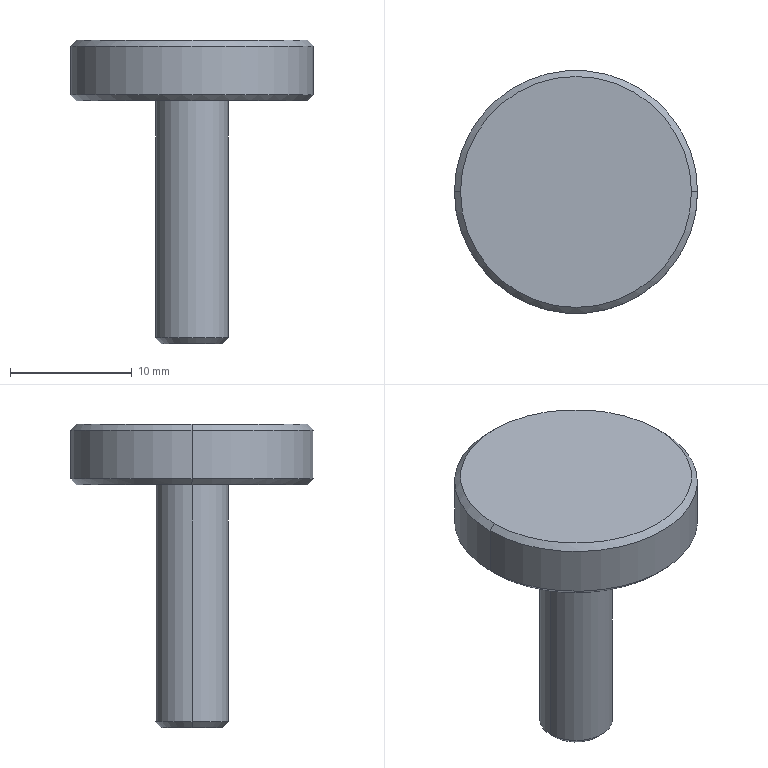Part | NX | features BREP 1 | 1 solid | 16 faces | box 20 x 20 x 25 mm | volume 2097 mm3 | cylinder 6 | cone 6 | plane 4 | commonest cylinder face diameters 3 x2 6 x2 20 x2
STEP:
#1=CARTESIAN_POINT('',(1.5,0.,3.));
#2=VERTEX_POINT('',#1);
#3=CARTESIAN_POINT('',(-1.5,0.,3.));
#4=VERTEX_POINT('',#3);
#5=CARTESIAN_POINT('',(0.,0.,3.));
#6=DIRECTION('',(0.,0.,-1.));
#7=DIRECTION('',(-1.,0.,0.));
#8=AXIS2_PLACEMENT_3D('',#5,#6,#7);
#9=CIRCLE('',#8,1.5);
#10=EDGE_CURVE('',#2,#4,#9,.T.);
#11=ORIENTED_EDGE('',*,*,#10,.F.);
#12=CARTESIAN_POINT('',(1.5,0.,0.));
#13=VERTEX_POINT('',#12);
#14=CARTESIAN_POINT('',(1.5,0.,3.));
#15=DIRECTION('',(0.,0.,-1.));
#16=VECTOR('',#15,1000.);
#17=LINE('',#14,#16);
#18=EDGE_CURVE('',#2,#13,#17,.T.);
#19=ORIENTED_EDGE('',*,*,#18,.T.);
#20=CARTESIAN_POINT('',(-1.5,0.,0.));
#21=VERTEX_POINT('',#20);
#22=CARTESIAN_POINT('',(0.,0.,0.));
#23=DIRECTION('',(0.,0.,-1.));
#24=DIRECTION('',(-1.,0.,0.));
#25=AXIS2_PLACEMENT_3D('',#22,#23,#24);
#26=CIRCLE('',#25,1.5);
#27=EDGE_CURVE('',#13,#21,#26,.T.);
#28=ORIENTED_EDGE('',*,*,#27,.T.);
#29=CARTESIAN_POINT('',(-1.5,0.,3.));
#30=DIRECTION('',(0.,0.,-1.));
#31=VECTOR('',#30,1000.);
#32=LINE('',#29,#31);
#33=EDGE_CURVE('',#4,#21,#32,.T.);
#34=ORIENTED_EDGE('',*,*,#33,.F.);
#35=EDGE_LOOP('',(#11,#19,#28,#34));
#36=FACE_BOUND('',#35,.T.);
#37=CARTESIAN_POINT('',(0.,0.,3.));
#38=DIRECTION('',(0.,0.,-1.));
#39=DIRECTION('',(-1.,0.,0.));
#40=AXIS2_PLACEMENT_3D('',#37,#38,#39);
#41=CYLINDRICAL_SURFACE('',#40,1.5);
#42=ADVANCED_FACE('',(#36),#41,.F.);
#43=CARTESIAN_POINT('',(-9.5,0.,20.));
#44=VERTEX_POINT('',#43);
#45=CARTESIAN_POINT('',(9.5,0.,20.));
#46=VERTEX_POINT('',#45);
#47=CARTESIAN_POINT('',(0.,0.,20.));
#48=DIRECTION('',(0.,0.,-1.));
#49=DIRECTION('',(1.,0.,0.));
#50=AXIS2_PLACEMENT_3D('',#47,#48,#49);
#51=CIRCLE('',#50,9.5);
#52=EDGE_CURVE('',#44,#46,#51,.T.);
#53=ORIENTED_EDGE('',*,*,#52,.F.);
#54=CARTESIAN_POINT('',(-10.,0.,20.5));
#55=VERTEX_POINT('',#54);
#56=CARTESIAN_POINT('',(-10.,0.,20.5));
#57=DIRECTION('',(-0.7071,0.,0.7071));
#58=VECTOR('',#57,1000.);
#59=LINE('',#56,#58);
#60=EDGE_CURVE('',#55,#44,#59,.F.);
#61=ORIENTED_EDGE('',*,*,#60,.F.);
#62=CARTESIAN_POINT('',(10.,0.,20.5));
#63=VERTEX_POINT('',#62);
#64=CARTESIAN_POINT('',(0.,0.,20.5));
#65=DIRECTION('',(0.,0.,1.));
#66=DIRECTION('',(1.,0.,0.));
#67=AXIS2_PLACEMENT_3D('',#64,#65,#66);
#68=CIRCLE('',#67,10.);
#69=EDGE_CURVE('',#63,#55,#68,.T.);
#70=ORIENTED_EDGE('',*,*,#69,.F.);
#71=CARTESIAN_POINT('',(10.,0.,20.5));
#72=DIRECTION('',(0.7071,0.,0.7071));
#73=VECTOR('',#72,1000.);
#74=LINE('',#71,#73);
#75=EDGE_CURVE('',#63,#46,#74,.F.);
#76=ORIENTED_EDGE('',*,*,#75,.T.);
#77=EDGE_LOOP('',(#53,#61,#70,#76));
#78=FACE_BOUND('',#77,.T.);
#79=CARTESIAN_POINT('',(0.,0.,20.5));
#80=DIRECTION('',(0.,0.,1.));
#81=DIRECTION('',(1.,0.,0.));
#82=AXIS2_PLACEMENT_3D('',#79,#80,#81);
#83=CONICAL_SURFACE('',#82,10.,0.7854);
#84=ADVANCED_FACE('',(#78),#83,.T.);
#85=CARTESIAN_POINT('',(9.5,0.,25.));
#86=VERTEX_POINT('',#85);
#87=CARTESIAN_POINT('',(-9.5,0.,25.));
#88=VERTEX_POINT('',#87);
#89=CARTESIAN_POINT('',(0.,0.,25.));
#90=DIRECTION('',(0.,0.,1.));
#91=DIRECTION('',(1.,0.,0.));
#92=AXIS2_PLACEMENT_3D('',#89,#90,#91);
#93=CIRCLE('',#92,9.5);
#94=EDGE_CURVE('',#86,#88,#93,.T.);
#95=ORIENTED_EDGE('',*,*,#94,.F.);
#96=CARTESIAN_POINT('',(10.,0.,24.5));
#97=VERTEX_POINT('',#96);
#98=CARTESIAN_POINT('',(9.5,0.,25.));
#99=DIRECTION('',(0.7071,0.,-0.7071));
#100=VECTOR('',#99,1000.);
#101=LINE('',#98,#100);
#102=EDGE_CURVE('',#86,#97,#101,.T.);
#103=ORIENTED_EDGE('',*,*,#102,.T.);
#104=CARTESIAN_POINT('',(-10.,0.,24.5));
#105=VERTEX_POINT('',#104);
#106=CARTESIAN_POINT('',(0.,0.,24.5));
#107=DIRECTION('',(0.,0.,-1.));
#108=DIRECTION('',(1.,0.,0.));
#109=AXIS2_PLACEMENT_3D('',#106,#107,#108);
#110=CIRCLE('',#109,10.);
#111=EDGE_CURVE('',#105,#97,#110,.T.);
#112=ORIENTED_EDGE('',*,*,#111,.F.);
#113=CARTESIAN_POINT('',(-9.5,0.,25.));
#114=DIRECTION('',(-0.7071,0.,-0.7071));
#115=VECTOR('',#114,1000.);
#116=LINE('',#113,#115);
#117=EDGE_CURVE('',#88,#105,#116,.T.);
#118=ORIENTED_EDGE('',*,*,#117,.F.);
#119=EDGE_LOOP('',(#95,#103,#112,#118));
#120=FACE_BOUND('',#119,.T.);
#121=CARTESIAN_POINT('',(0.,0.,25.));
#122=DIRECTION('',(0.,0.,-1.));
#123=DIRECTION('',(-1.,0.,0.));
#124=AXIS2_PLACEMENT_3D('',#121,#122,#123);
#125=CONICAL_SURFACE('',#124,9.5,0.7854);
#126=ADVANCED_FACE('',(#120),#125,.T.);
#127=CARTESIAN_POINT('',(-2.5,0.,0.));
#128=VERTEX_POINT('',#127);
#129=CARTESIAN_POINT('',(2.5,0.,0.));
#130=VERTEX_POINT('',#129);
#131=CARTESIAN_POINT('',(0.,0.,0.));
#132=DIRECTION('',(0.,0.,-1.));
#133=DIRECTION('',(1.,0.,0.));
#134=AXIS2_PLACEMENT_3D('',#131,#132,#133);
#135=CIRCLE('',#134,2.5);
#136=EDGE_CURVE('',#128,#130,#135,.T.);
#137=ORIENTED_EDGE('',*,*,#136,.F.);
#138=CARTESIAN_POINT('',(-3.,0.,0.5));
#139=VERTEX_POINT('',#138);
#140=CARTESIAN_POINT('',(-3.,0.,0.5));
#141=DIRECTION('',(-0.7071,0.,0.7071));
#142=VECTOR('',#141,1000.);
#143=LINE('',#140,#142);
#144=EDGE_CURVE('',#139,#128,#143,.F.);
#145=ORIENTED_EDGE('',*,*,#144,.F.);
#146=CARTESIAN_POINT('',(3.,0.,0.5));
#147=VERTEX_POINT('',#146);
#148=CARTESIAN_POINT('',(0.,0.,0.5));
#149=DIRECTION('',(0.,0.,1.));
#150=DIRECTION('',(1.,0.,0.));
#151=AXIS2_PLACEMENT_3D('',#148,#149,#150);
#152=CIRCLE('',#151,3.);
#153=EDGE_CURVE('',#147,#139,#152,.T.);
#154=ORIENTED_EDGE('',*,*,#153,.F.);
#155=CARTESIAN_POINT('',(3.,0.,0.5));
#156=DIRECTION('',(0.7071,0.,0.7071));
#157=VECTOR('',#156,1000.);
#158=LINE('',#155,#157);
#159=EDGE_CURVE('',#147,#130,#158,.F.);
#160=ORIENTED_EDGE('',*,*,#159,.T.);
#161=EDGE_LOOP('',(#137,#145,#154,#160));
#162=FACE_BOUND('',#161,.T.);
#163=CARTESIAN_POINT('',(0.,0.,0.5));
#164=DIRECTION('',(0.,0.,1.));
#165=DIRECTION('',(1.,0.,0.));
#166=AXIS2_PLACEMENT_3D('',#163,#164,#165);
#167=CONICAL_SURFACE('',#166,3.,0.7854);
#168=ADVANCED_FACE('',(#162),#167,.T.);
#169=ORIENTED_EDGE('',*,*,#111,.T.);
#170=CARTESIAN_POINT('',(10.,0.,25.));
#171=DIRECTION('',(0.,0.,-1.));
#172=VECTOR('',#171,1000.);
#173=LINE('',#170,#172);
#174=EDGE_CURVE('',#97,#63,#173,.T.);
#175=ORIENTED_EDGE('',*,*,#174,.T.);
#176=ORIENTED_EDGE('',*,*,#69,.T.);
#177=CARTESIAN_POINT('',(-10.,0.,25.));
#178=DIRECTION('',(0.,0.,-1.));
#179=VECTOR('',#178,1000.);
#180=LINE('',#177,#179);
#181=EDGE_CURVE('',#105,#55,#180,.T.);
#182=ORIENTED_EDGE('',*,*,#181,.F.);
#183=EDGE_LOOP('',(#169,#175,#176,#182));
#184=FACE_BOUND('',#183,.T.);
#185=CARTESIAN_POINT('',(0.,0.,25.));
#186=DIRECTION('',(0.,0.,-1.));
#187=DIRECTION('',(-1.,0.,0.));
#188=AXIS2_PLACEMENT_3D('',#185,#186,#187);
#189=CYLINDRICAL_SURFACE('',#188,10.);
#190=ADVANCED_FACE('',(#184),#189,.T.);
#191=CARTESIAN_POINT('',(3.,0.,20.));
#192=VERTEX_POINT('',#191);
#193=CARTESIAN_POINT('',(-3.,0.,20.));
#194=VERTEX_POINT('',#193);
#195=CARTESIAN_POINT('',(0.,0.,20.));
#196=DIRECTION('',(0.,0.,1.));
#197=DIRECTION('',(1.,0.,0.));
#198=AXIS2_PLACEMENT_3D('',#195,#196,#197);
#199=CIRCLE('',#198,3.);
#200=EDGE_CURVE('',#192,#194,#199,.T.);
#201=ORIENTED_EDGE('',*,*,#200,.F.);
#202=CARTESIAN_POINT('',(3.,0.,20.));
#203=DIRECTION('',(0.,0.,-1.));
#204=VECTOR('',#203,1000.);
#205=LINE('',#202,#204);
#206=EDGE_CURVE('',#192,#147,#205,.T.);
#207=ORIENTED_EDGE('',*,*,#206,.T.);
#208=ORIENTED_EDGE('',*,*,#153,.T.);
#209=CARTESIAN_POINT('',(-3.,0.,20.));
#210=DIRECTION('',(0.,0.,-1.));
#211=VECTOR('',#210,1000.);
#212=LINE('',#209,#211);
#213=EDGE_CURVE('',#194,#139,#212,.T.);
#214=ORIENTED_EDGE('',*,*,#213,.F.);
#215=EDGE_LOOP('',(#201,#207,#208,#214));
#216=FACE_BOUND('',#215,.T.);
#217=CARTESIAN_POINT('',(0.,0.,20.));
#218=DIRECTION('',(0.,0.,-1.));
#219=DIRECTION('',(-1.,0.,0.));
#220=AXIS2_PLACEMENT_3D('',#217,#218,#219);
#221=CYLINDRICAL_SURFACE('',#220,3.);
#222=ADVANCED_FACE('',(#216),#221,.T.);
#223=ORIENTED_EDGE('',*,*,#206,.F.);
#224=CARTESIAN_POINT('',(0.,0.,20.));
#225=DIRECTION('',(0.,0.,1.));
#226=DIRECTION('',(1.,0.,0.));
#227=AXIS2_PLACEMENT_3D('',#224,#225,#226);
#228=CIRCLE('',#227,3.);
#229=EDGE_CURVE('',#194,#192,#228,.T.);
#230=ORIENTED_EDGE('',*,*,#229,.F.);
#231=ORIENTED_EDGE('',*,*,#213,.T.);
#232=CARTESIAN_POINT('',(0.,0.,0.5));
#233=DIRECTION('',(0.,0.,1.));
#234=DIRECTION('',(1.,0.,0.));
#235=AXIS2_PLACEMENT_3D('',#232,#233,#234);
#236=CIRCLE('',#235,3.);
#237=EDGE_CURVE('',#139,#147,#236,.T.);
#238=ORIENTED_EDGE('',*,*,#237,.T.);
#239=EDGE_LOOP('',(#223,#230,#231,#238));
#240=FACE_BOUND('',#239,.T.);
#241=CARTESIAN_POINT('',(0.,0.,20.));
#242=DIRECTION('',(0.,0.,-1.));
#243=DIRECTION('',(-1.,0.,0.));
#244=AXIS2_PLACEMENT_3D('',#241,#242,#243);
#245=CYLINDRICAL_SURFACE('',#244,3.);
#246=ADVANCED_FACE('',(#240),#245,.T.);
#247=CARTESIAN_POINT('',(0.,0.,0.));
#248=DIRECTION('',(0.,0.,-1.));
#249=DIRECTION('',(1.,0.,0.));
#250=AXIS2_PLACEMENT_3D('',#247,#248,#249);
#251=CIRCLE('',#250,2.5);
#252=EDGE_CURVE('',#130,#128,#251,.T.);
#253=ORIENTED_EDGE('',*,*,#252,.T.);
#254=ORIENTED_EDGE('',*,*,#136,.T.);
#255=EDGE_LOOP('',(#253,#254));
#256=FACE_BOUND('',#255,.T.);
#257=CARTESIAN_POINT('',(0.,0.,0.));
#258=DIRECTION('',(0.,0.,-1.));
#259=DIRECTION('',(-1.,0.,0.));
#260=AXIS2_PLACEMENT_3D('',#257,#258,#259);
#261=CIRCLE('',#260,1.5);
#262=EDGE_CURVE('',#21,#13,#261,.T.);
#263=ORIENTED_EDGE('',*,*,#262,.F.);
#264=ORIENTED_EDGE('',*,*,#27,.F.);
#265=EDGE_LOOP('',(#263,#264));
#266=FACE_BOUND('',#265,.T.);
#267=CARTESIAN_POINT('',(0.,0.,0.));
#268=DIRECTION('',(0.,0.,1.));
#269=DIRECTION('',(1.,0.,0.));
#270=AXIS2_PLACEMENT_3D('',#267,#268,#269);
#271=PLANE('',#270);
#272=ADVANCED_FACE('',(#256,#266),#271,.F.);
#273=CARTESIAN_POINT('',(0.,0.,20.));
#274=DIRECTION('',(0.,0.,-1.));
#275=DIRECTION('',(1.,0.,0.));
#276=AXIS2_PLACEMENT_3D('',#273,#274,#275);
#277=CIRCLE('',#276,9.5);
#278=EDGE_CURVE('',#46,#44,#277,.T.);
#279=ORIENTED_EDGE('',*,*,#278,.T.);
#280=ORIENTED_EDGE('',*,*,#52,.T.);
#281=EDGE_LOOP('',(#279,#280));
#282=FACE_BOUND('',#281,.T.);
#283=ORIENTED_EDGE('',*,*,#229,.T.);
#284=ORIENTED_EDGE('',*,*,#200,.T.);
#285=EDGE_LOOP('',(#283,#284));
#286=FACE_BOUND('',#285,.T.);
#287=CARTESIAN_POINT('',(0.,0.,20.));
#288=DIRECTION('',(0.,0.,1.));
#289=DIRECTION('',(1.,0.,0.));
#290=AXIS2_PLACEMENT_3D('',#287,#288,#289);
#291=PLANE('',#290);
#292=ADVANCED_FACE('',(#282,#286),#291,.F.);
#293=ORIENTED_EDGE('',*,*,#174,.F.);
#294=CARTESIAN_POINT('',(0.,0.,24.5));
#295=DIRECTION('',(0.,0.,-1.));
#296=DIRECTION('',(1.,0.,0.));
#297=AXIS2_PLACEMENT_3D('',#294,#295,#296);
#298=CIRCLE('',#297,10.);
#299=EDGE_CURVE('',#97,#105,#298,.T.);
#300=ORIENTED_EDGE('',*,*,#299,.T.);
#301=ORIENTED_EDGE('',*,*,#181,.T.);
#302=CARTESIAN_POINT('',(0.,0.,20.5));
#303=DIRECTION('',(0.,0.,1.));
#304=DIRECTION('',(1.,0.,0.));
#305=AXIS2_PLACEMENT_3D('',#302,#303,#304);
#306=CIRCLE('',#305,10.);
#307=EDGE_CURVE('',#55,#63,#306,.T.);
#308=ORIENTED_EDGE('',*,*,#307,.T.);
#309=EDGE_LOOP('',(#293,#300,#301,#308));
#310=FACE_BOUND('',#309,.T.);
#311=CARTESIAN_POINT('',(0.,0.,25.));
#312=DIRECTION('',(0.,0.,-1.));
#313=DIRECTION('',(-1.,0.,0.));
#314=AXIS2_PLACEMENT_3D('',#311,#312,#313);
#315=CYLINDRICAL_SURFACE('',#314,10.);
#316=ADVANCED_FACE('',(#310),#315,.T.);
#317=CARTESIAN_POINT('',(0.,0.,25.));
#318=DIRECTION('',(0.,0.,1.));
#319=DIRECTION('',(1.,0.,0.));
#320=AXIS2_PLACEMENT_3D('',#317,#318,#319);
#321=CIRCLE('',#320,9.5);
#322=EDGE_CURVE('',#88,#86,#321,.T.);
#323=ORIENTED_EDGE('',*,*,#322,.T.);
#324=ORIENTED_EDGE('',*,*,#94,.T.);
#325=EDGE_LOOP('',(#323,#324));
#326=FACE_BOUND('',#325,.T.);
#327=CARTESIAN_POINT('',(0.,0.,25.));
#328=DIRECTION('',(0.,0.,1.));
#329=DIRECTION('',(1.,0.,0.));
#330=AXIS2_PLACEMENT_3D('',#327,#328,#329);
#331=PLANE('',#330);
#332=ADVANCED_FACE('',(#326),#331,.T.);
#333=ORIENTED_EDGE('',*,*,#144,.T.);
#334=ORIENTED_EDGE('',*,*,#252,.F.);
#335=ORIENTED_EDGE('',*,*,#159,.F.);
#336=ORIENTED_EDGE('',*,*,#237,.F.);
#337=EDGE_LOOP('',(#333,#334,#335,#336));
#338=FACE_BOUND('',#337,.T.);
#339=CARTESIAN_POINT('',(0.,0.,0.5));
#340=DIRECTION('',(0.,0.,1.));
#341=DIRECTION('',(1.,0.,0.));
#342=AXIS2_PLACEMENT_3D('',#339,#340,#341);
#343=CONICAL_SURFACE('',#342,3.,0.7854);
#344=ADVANCED_FACE('',(#338),#343,.T.);
#345=ORIENTED_EDGE('',*,*,#102,.F.);
#346=ORIENTED_EDGE('',*,*,#322,.F.);
#347=ORIENTED_EDGE('',*,*,#117,.T.);
#348=ORIENTED_EDGE('',*,*,#299,.F.);
#349=EDGE_LOOP('',(#345,#346,#347,#348));
#350=FACE_BOUND('',#349,.T.);
#351=CARTESIAN_POINT('',(0.,0.,25.));
#352=DIRECTION('',(0.,0.,-1.));
#353=DIRECTION('',(-1.,0.,0.));
#354=AXIS2_PLACEMENT_3D('',#351,#352,#353);
#355=CONICAL_SURFACE('',#354,9.5,0.7854);
#356=ADVANCED_FACE('',(#350),#355,.T.);
#357=ORIENTED_EDGE('',*,*,#60,.T.);
#358=ORIENTED_EDGE('',*,*,#278,.F.);
#359=ORIENTED_EDGE('',*,*,#75,.F.);
#360=ORIENTED_EDGE('',*,*,#307,.F.);
#361=EDGE_LOOP('',(#357,#358,#359,#360));
#362=FACE_BOUND('',#361,.T.);
#363=CARTESIAN_POINT('',(0.,0.,20.5));
#364=DIRECTION('',(0.,0.,1.));
#365=DIRECTION('',(1.,0.,0.));
#366=AXIS2_PLACEMENT_3D('',#363,#364,#365);
#367=CONICAL_SURFACE('',#366,10.,0.7854);
#368=ADVANCED_FACE('',(#362),#367,.T.);
#369=ORIENTED_EDGE('',*,*,#18,.F.);
#370=CARTESIAN_POINT('',(0.,0.,3.));
#371=DIRECTION('',(0.,0.,-1.));
#372=DIRECTION('',(-1.,0.,0.));
#373=AXIS2_PLACEMENT_3D('',#370,#371,#372);
#374=CIRCLE('',#373,1.5);
#375=EDGE_CURVE('',#4,#2,#374,.T.);
#376=ORIENTED_EDGE('',*,*,#375,.F.);
#377=ORIENTED_EDGE('',*,*,#33,.T.);
#378=ORIENTED_EDGE('',*,*,#262,.T.);
#379=EDGE_LOOP('',(#369,#376,#377,#378));
#380=FACE_BOUND('',#379,.T.);
#381=CARTESIAN_POINT('',(0.,0.,3.));
#382=DIRECTION('',(0.,0.,-1.));
#383=DIRECTION('',(-1.,0.,0.));
#384=AXIS2_PLACEMENT_3D('',#381,#382,#383);
#385=CYLINDRICAL_SURFACE('',#384,1.5);
#386=ADVANCED_FACE('',(#380),#385,.F.);
#387=ORIENTED_EDGE('',*,*,#375,.T.);
#388=ORIENTED_EDGE('',*,*,#10,.T.);
#389=EDGE_LOOP('',(#387,#388));
#390=FACE_BOUND('',#389,.T.);
#391=CARTESIAN_POINT('',(0.,0.,3.));
#392=DIRECTION('',(0.,0.,-1.));
#393=DIRECTION('',(0.,-1.,0.));
#394=AXIS2_PLACEMENT_3D('',#391,#392,#393);
#395=PLANE('',#394);
#396=ADVANCED_FACE('',(#390),#395,.T.);
#397=CLOSED_SHELL('',(#42,#84,#126,#168,#190,#222,#246,#272,#292,#316,#332,#344,#356,#368,#386,#396));
#398=MANIFOLD_SOLID_BREP('',#397);
#399=(LENGTH_UNIT()NAMED_UNIT(*)SI_UNIT(.MILLI.,.METRE.));
#400=UNCERTAINTY_MEASURE_WITH_UNIT(LENGTH_MEASURE(0.00001),#399,'','');
#401=(NAMED_UNIT(*)PLANE_ANGLE_UNIT()SI_UNIT($,.RADIAN.));
#402=(NAMED_UNIT(*)SI_UNIT($,.STERADIAN.)SOLID_ANGLE_UNIT());
#403=(GEOMETRIC_REPRESENTATION_CONTEXT(3)GLOBAL_UNCERTAINTY_ASSIGNED_CONTEXT((#400))GLOBAL_UNIT_ASSIGNED_CONTEXT((#399,#401,#402))REPRESENTATION_CONTEXT('',''));
#404=ADVANCED_BREP_SHAPE_REPRESENTATION('',(#398),#403);